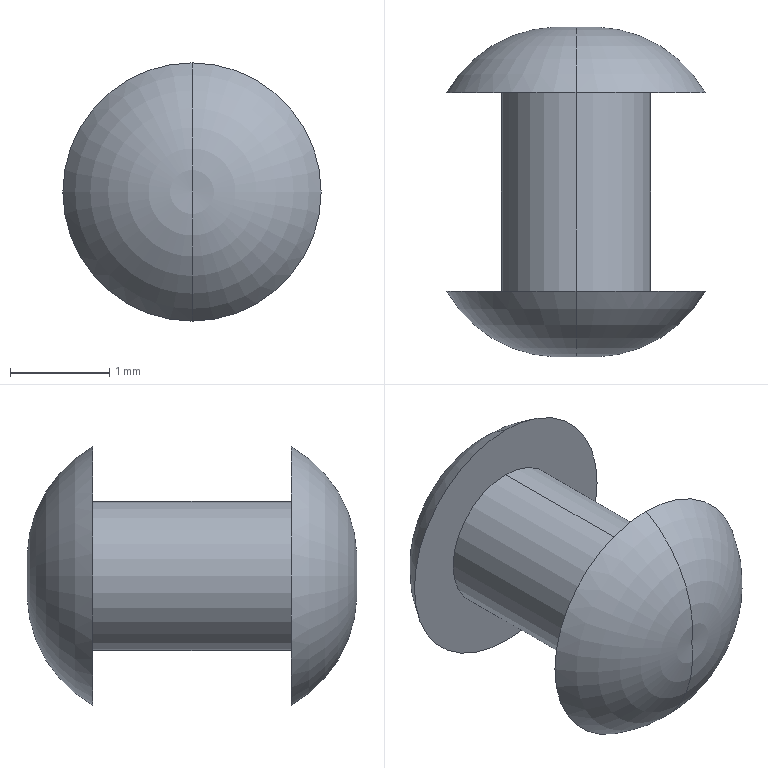Part | STEP file | Szegecs | 1 solid | 8 faces | box 2.6 x 3.322 x 2.6 mm | volume 7.735 mm3 | torus 4 | cylinder 2 | plane 2 | commonest cylinder face diameters 1.5 x2
STEP:
#1=CARTESIAN_POINT('',(0.,-2.,0.75));
#2=VERTEX_POINT('',#1);
#3=CARTESIAN_POINT('',(0.,-2.,-0.75));
#4=VERTEX_POINT('',#3);
#5=CARTESIAN_POINT('',(0.,-2.,0.));
#6=DIRECTION('',(0.,1.,0.));
#7=DIRECTION('',(0.,0.,1.));
#8=AXIS2_PLACEMENT_3D('',#5,#6,#7);
#9=CIRCLE('',#8,0.75);
#10=EDGE_CURVE('',#2,#4,#9,.T.);
#11=ORIENTED_EDGE('',*,*,#10,.T.);
#12=CARTESIAN_POINT('',(0.,0.,-0.75));
#13=VERTEX_POINT('',#12);
#14=CARTESIAN_POINT('',(0.,-2.,-0.75));
#15=DIRECTION('',(0.,1.,0.));
#16=VECTOR('',#15,1000.);
#17=LINE('',#14,#16);
#18=EDGE_CURVE('',#4,#13,#17,.T.);
#19=ORIENTED_EDGE('',*,*,#18,.T.);
#20=CARTESIAN_POINT('',(0.,0.,0.75));
#21=VERTEX_POINT('',#20);
#22=CARTESIAN_POINT('',(0.,0.,0.));
#23=DIRECTION('',(0.,-1.,0.));
#24=DIRECTION('',(0.,0.,1.));
#25=AXIS2_PLACEMENT_3D('',#22,#23,#24);
#26=CIRCLE('',#25,0.75);
#27=EDGE_CURVE('',#13,#21,#26,.T.);
#28=ORIENTED_EDGE('',*,*,#27,.T.);
#29=CARTESIAN_POINT('',(0.,-2.,0.75));
#30=DIRECTION('',(0.,1.,0.));
#31=VECTOR('',#30,1000.);
#32=LINE('',#29,#31);
#33=EDGE_CURVE('',#2,#21,#32,.T.);
#34=ORIENTED_EDGE('',*,*,#33,.F.);
#35=EDGE_LOOP('',(#11,#19,#28,#34));
#36=FACE_OUTER_BOUND('',#35,.T.);
#37=CARTESIAN_POINT('',(0.,-2.,0.));
#38=DIRECTION('',(0.,1.,0.));
#39=DIRECTION('',(0.,0.,1.));
#40=AXIS2_PLACEMENT_3D('',#37,#38,#39);
#41=CYLINDRICAL_SURFACE('',#40,0.75);
#42=ADVANCED_FACE('',(#36),#41,.T.);
#43=CARTESIAN_POINT('',(0.,0.,-1.3));
#44=VERTEX_POINT('',#43);
#45=CARTESIAN_POINT('',(0.,0.,1.3));
#46=VERTEX_POINT('',#45);
#47=CARTESIAN_POINT('',(0.,0.,0.));
#48=DIRECTION('',(0.,-1.,0.));
#49=DIRECTION('',(0.,0.,1.));
#50=AXIS2_PLACEMENT_3D('',#47,#48,#49);
#51=CIRCLE('',#50,1.3);
#52=EDGE_CURVE('',#44,#46,#51,.T.);
#53=ORIENTED_EDGE('',*,*,#52,.F.);
#54=CARTESIAN_POINT('',(0.,0.65,0.));
#55=VERTEX_POINT('',#54);
#56=CARTESIAN_POINT('',(0.,-0.6391,-0.1679));
#57=DIRECTION('',(1.,0.,0.));
#58=DIRECTION('',(0.,0.,-1.));
#59=AXIS2_PLACEMENT_3D('',#56,#57,#58);
#60=CIRCLE('',#59,1.3);
#61=EDGE_CURVE('',#44,#55,#60,.T.);
#62=ORIENTED_EDGE('',*,*,#61,.T.);
#63=CARTESIAN_POINT('',(0.,-0.6391,0.1679));
#64=DIRECTION('',(-1.,0.,0.));
#65=DIRECTION('',(0.,0.,1.));
#66=AXIS2_PLACEMENT_3D('',#63,#64,#65);
#67=CIRCLE('',#66,1.3);
#68=EDGE_CURVE('',#46,#55,#67,.T.);
#69=ORIENTED_EDGE('',*,*,#68,.F.);
#70=EDGE_LOOP('',(#53,#62,#69));
#71=FACE_OUTER_BOUND('',#70,.T.);
#72=CARTESIAN_POINT('',(0.,-0.6391,0.));
#73=DIRECTION('',(0.,1.,0.));
#74=DIRECTION('',(0.,0.,1.));
#75=AXIS2_PLACEMENT_3D('',#72,#73,#74);
#76=TOROIDAL_SURFACE('',#75,0.1679,1.3);
#77=ADVANCED_FACE('',(#71),#76,.T.);
#78=CARTESIAN_POINT('',(0.,-2.65,0.));
#79=VERTEX_POINT('',#78);
#80=CARTESIAN_POINT('',(0.,-2.,1.3));
#81=VERTEX_POINT('',#80);
#82=CARTESIAN_POINT('',(0.,-1.361,0.1679));
#83=DIRECTION('',(-1.,0.,0.));
#84=DIRECTION('',(0.,0.,1.));
#85=AXIS2_PLACEMENT_3D('',#82,#83,#84);
#86=CIRCLE('',#85,1.3);
#87=EDGE_CURVE('',#79,#81,#86,.T.);
#88=ORIENTED_EDGE('',*,*,#87,.F.);
#89=CARTESIAN_POINT('',(0.,-2.,-1.3));
#90=VERTEX_POINT('',#89);
#91=CARTESIAN_POINT('',(0.,-1.361,-0.1679));
#92=DIRECTION('',(1.,0.,0.));
#93=DIRECTION('',(0.,0.,-1.));
#94=AXIS2_PLACEMENT_3D('',#91,#92,#93);
#95=CIRCLE('',#94,1.3);
#96=EDGE_CURVE('',#79,#90,#95,.T.);
#97=ORIENTED_EDGE('',*,*,#96,.T.);
#98=CARTESIAN_POINT('',(0.,-2.,0.));
#99=DIRECTION('',(0.,-1.,0.));
#100=DIRECTION('',(0.,0.,1.));
#101=AXIS2_PLACEMENT_3D('',#98,#99,#100);
#102=CIRCLE('',#101,1.3);
#103=EDGE_CURVE('',#90,#81,#102,.T.);
#104=ORIENTED_EDGE('',*,*,#103,.T.);
#105=EDGE_LOOP('',(#88,#97,#104));
#106=FACE_OUTER_BOUND('',#105,.T.);
#107=CARTESIAN_POINT('',(0.,-1.361,0.));
#108=DIRECTION('',(0.,1.,0.));
#109=DIRECTION('',(0.,0.,1.));
#110=AXIS2_PLACEMENT_3D('',#107,#108,#109);
#111=TOROIDAL_SURFACE('',#110,0.1679,1.3);
#112=ADVANCED_FACE('',(#106),#111,.T.);
#113=ORIENTED_EDGE('',*,*,#18,.F.);
#114=CARTESIAN_POINT('',(0.,-2.,0.));
#115=DIRECTION('',(0.,1.,0.));
#116=DIRECTION('',(0.,0.,1.));
#117=AXIS2_PLACEMENT_3D('',#114,#115,#116);
#118=CIRCLE('',#117,0.75);
#119=EDGE_CURVE('',#4,#2,#118,.T.);
#120=ORIENTED_EDGE('',*,*,#119,.T.);
#121=ORIENTED_EDGE('',*,*,#33,.T.);
#122=CARTESIAN_POINT('',(0.,0.,0.));
#123=DIRECTION('',(0.,-1.,0.));
#124=DIRECTION('',(0.,0.,1.));
#125=AXIS2_PLACEMENT_3D('',#122,#123,#124);
#126=CIRCLE('',#125,0.75);
#127=EDGE_CURVE('',#21,#13,#126,.T.);
#128=ORIENTED_EDGE('',*,*,#127,.T.);
#129=EDGE_LOOP('',(#113,#120,#121,#128));
#130=FACE_OUTER_BOUND('',#129,.T.);
#131=CARTESIAN_POINT('',(0.,-2.,0.));
#132=DIRECTION('',(0.,1.,0.));
#133=DIRECTION('',(0.,0.,1.));
#134=AXIS2_PLACEMENT_3D('',#131,#132,#133);
#135=CYLINDRICAL_SURFACE('',#134,0.75);
#136=ADVANCED_FACE('',(#130),#135,.T.);
#137=CARTESIAN_POINT('',(0.,0.,0.));
#138=DIRECTION('',(0.,-1.,0.));
#139=DIRECTION('',(0.,0.,1.));
#140=AXIS2_PLACEMENT_3D('',#137,#138,#139);
#141=CIRCLE('',#140,1.3);
#142=EDGE_CURVE('',#46,#44,#141,.T.);
#143=ORIENTED_EDGE('',*,*,#142,.T.);
#144=ORIENTED_EDGE('',*,*,#52,.T.);
#145=EDGE_LOOP('',(#143,#144));
#146=FACE_OUTER_BOUND('',#145,.T.);
#147=ORIENTED_EDGE('',*,*,#127,.F.);
#148=ORIENTED_EDGE('',*,*,#27,.F.);
#149=EDGE_LOOP('',(#147,#148));
#150=FACE_BOUND('',#149,.T.);
#151=CARTESIAN_POINT('',(0.,0.,0.));
#152=DIRECTION('',(0.,-1.,0.));
#153=DIRECTION('',(0.,0.,-1.));
#154=AXIS2_PLACEMENT_3D('',#151,#152,#153);
#155=PLANE('',#154);
#156=ADVANCED_FACE('',(#146,#150),#155,.T.);
#157=CARTESIAN_POINT('',(0.,-2.,0.));
#158=DIRECTION('',(0.,-1.,0.));
#159=DIRECTION('',(0.,0.,1.));
#160=AXIS2_PLACEMENT_3D('',#157,#158,#159);
#161=CIRCLE('',#160,1.3);
#162=EDGE_CURVE('',#81,#90,#161,.T.);
#163=ORIENTED_EDGE('',*,*,#162,.F.);
#164=ORIENTED_EDGE('',*,*,#103,.F.);
#165=EDGE_LOOP('',(#163,#164));
#166=FACE_OUTER_BOUND('',#165,.T.);
#167=ORIENTED_EDGE('',*,*,#10,.F.);
#168=ORIENTED_EDGE('',*,*,#119,.F.);
#169=EDGE_LOOP('',(#167,#168));
#170=FACE_BOUND('',#169,.T.);
#171=CARTESIAN_POINT('',(0.,-2.,0.));
#172=DIRECTION('',(0.,-1.,0.));
#173=DIRECTION('',(0.,0.,-1.));
#174=AXIS2_PLACEMENT_3D('',#171,#172,#173);
#175=PLANE('',#174);
#176=ADVANCED_FACE('',(#166,#170),#175,.F.);
#177=ORIENTED_EDGE('',*,*,#61,.F.);
#178=ORIENTED_EDGE('',*,*,#142,.F.);
#179=ORIENTED_EDGE('',*,*,#68,.T.);
#180=EDGE_LOOP('',(#177,#178,#179));
#181=FACE_OUTER_BOUND('',#180,.T.);
#182=CARTESIAN_POINT('',(0.,-0.6391,0.));
#183=DIRECTION('',(0.,1.,0.));
#184=DIRECTION('',(0.,0.,1.));
#185=AXIS2_PLACEMENT_3D('',#182,#183,#184);
#186=TOROIDAL_SURFACE('',#185,0.1679,1.3);
#187=ADVANCED_FACE('',(#181),#186,.T.);
#188=ORIENTED_EDGE('',*,*,#96,.F.);
#189=ORIENTED_EDGE('',*,*,#87,.T.);
#190=ORIENTED_EDGE('',*,*,#162,.T.);
#191=EDGE_LOOP('',(#188,#189,#190));
#192=FACE_OUTER_BOUND('',#191,.T.);
#193=CARTESIAN_POINT('',(0.,-1.361,0.));
#194=DIRECTION('',(0.,1.,0.));
#195=DIRECTION('',(0.,0.,1.));
#196=AXIS2_PLACEMENT_3D('',#193,#194,#195);
#197=TOROIDAL_SURFACE('',#196,0.1679,1.3);
#198=ADVANCED_FACE('',(#192),#197,.T.);
#199=CLOSED_SHELL('',(#42,#77,#112,#136,#156,#176,#187,#198));
#200=MANIFOLD_SOLID_BREP('',#199);
#201=CARTESIAN_POINT('',(0.,0.,0.));
#202=DIRECTION('',(0.,0.,1.));
#203=DIRECTION('',(1.,0.,0.));
#204=AXIS2_PLACEMENT_3D('',#201,#202,#203);
#205=(LENGTH_UNIT()NAMED_UNIT(*)SI_UNIT(.MILLI.,.METRE.));
#206=UNCERTAINTY_MEASURE_WITH_UNIT(LENGTH_MEASURE(0.00001),#205,'','');
#207=(NAMED_UNIT(*)PLANE_ANGLE_UNIT()SI_UNIT($,.RADIAN.));
#208=(NAMED_UNIT(*)SI_UNIT($,.STERADIAN.)SOLID_ANGLE_UNIT());
#209=(GEOMETRIC_REPRESENTATION_CONTEXT(3)GLOBAL_UNCERTAINTY_ASSIGNED_CONTEXT((#206))GLOBAL_UNIT_ASSIGNED_CONTEXT((#205,#207,#208))REPRESENTATION_CONTEXT('',''));
#210=ADVANCED_BREP_SHAPE_REPRESENTATION('',(#200,#204),#209);